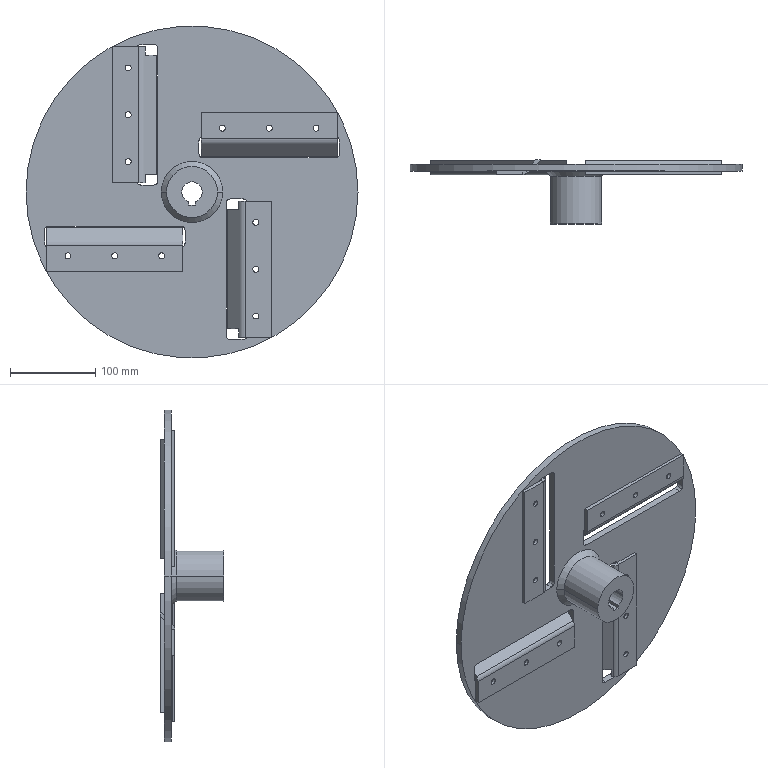Part | SolidWorks | features AEMSimFeature 1 | 8 solids | 218 faces | box 390 x 75.007 x 390 mm | volume 1088681 mm3 | cylinder 105 | plane 83 | cone 30 | commonest cylinder face diameters 7 x48 10 x32 55 x6 8 x4 16 x4 60 x4